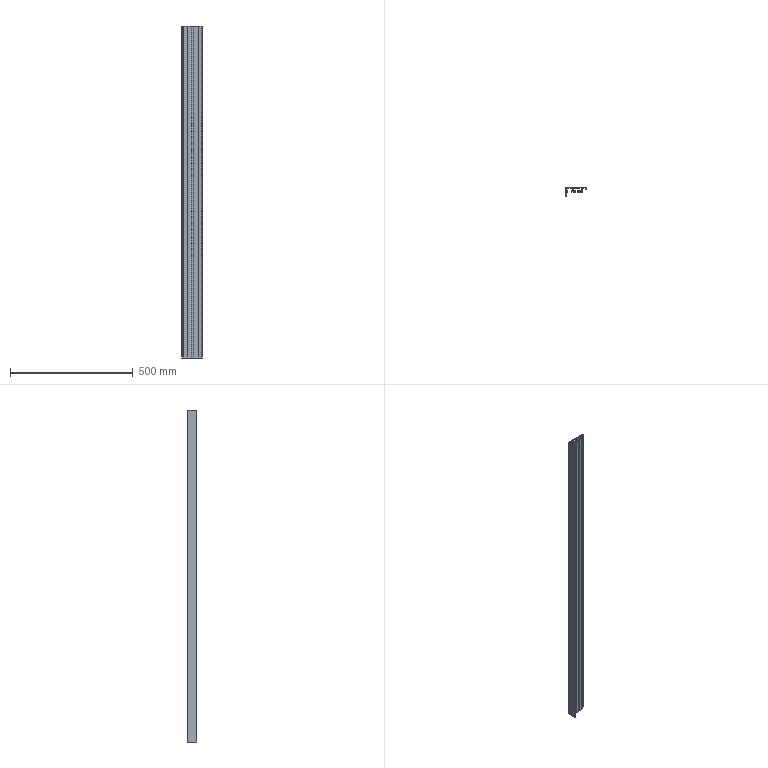Part | STEP file | SIDE-D default | 1 solid | 292 faces | box 82 x 38 x 1350 mm | volume 698294 mm3 | plane 257 | cylinder 35 | commonest cylinder face diameters 0.6 x18 1 x7 2 x4 3 x2 0.4 x1 4 x1